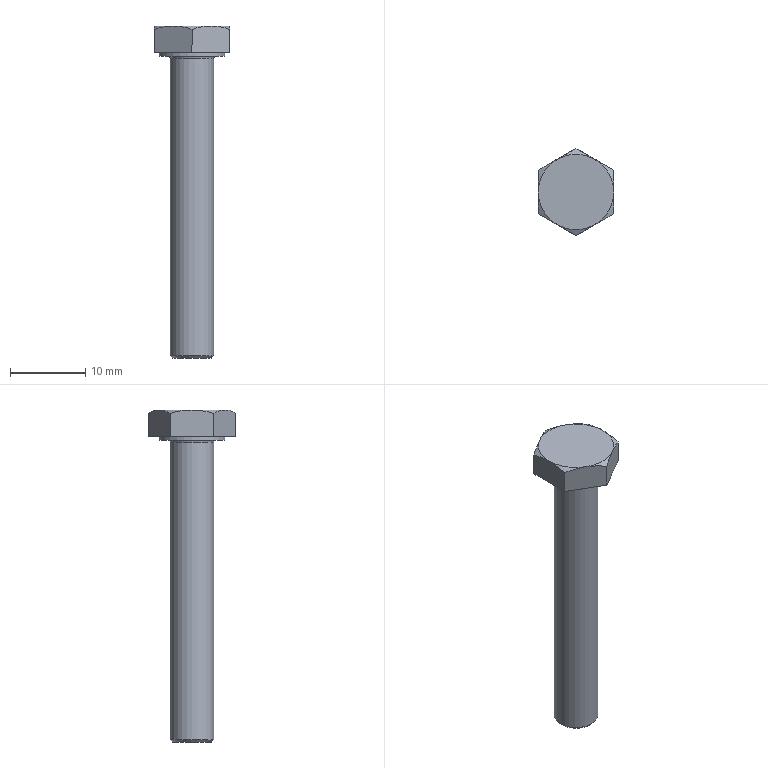Part | NX | features SKETCH 4, EXTRUDE 3, META 3, DATUM_CSYS 2, BLEND 1, CHAMFER 1, LINE 1, SWP104 1, SYMBOLIC_THREAD 1, THREADS 1 | 1 solid | 20 faces | box 10 x 11.547 x 44 mm | volume 1387 mm3 | plane 10 | cone 7 | cylinder 2 | torus 1 | commonest cylinder face diameters 5.795 x1 8.74 x1
STEP:
#1=CARTESIAN_POINT('',(3.147,0.,0.));
#2=VERTEX_POINT('',#1);
#3=CARTESIAN_POINT('',(0.,0.,0.));
#4=DIRECTION('',(0.,0.,1.));
#5=DIRECTION('',(1.,0.,0.));
#6=AXIS2_PLACEMENT_3D('',#3,#4,#5);
#7=CIRCLE('',#6,3.147);
#8=EDGE_CURVE('',#2,#2,#7,.T.);
#9=ORIENTED_EDGE('',*,*,#8,.T.);
#10=EDGE_LOOP('',(#9));
#11=FACE_BOUND('',#10,.T.);
#12=CARTESIAN_POINT('',(4.37,0.,0.));
#13=VERTEX_POINT('',#12);
#14=CARTESIAN_POINT('',(0.,0.,0.));
#15=DIRECTION('',(0.,0.,1.));
#16=DIRECTION('',(1.,0.,0.));
#17=AXIS2_PLACEMENT_3D('',#14,#15,#16);
#18=CIRCLE('',#17,4.37);
#19=EDGE_CURVE('',#13,#13,#18,.T.);
#20=ORIENTED_EDGE('',*,*,#19,.F.);
#21=EDGE_LOOP('',(#20));
#22=FACE_BOUND('',#21,.T.);
#23=CARTESIAN_POINT('',(0.,0.,0.));
#24=DIRECTION('',(0.,0.,1.));
#25=DIRECTION('',(1.,0.,0.));
#26=AXIS2_PLACEMENT_3D('',#23,#24,#25);
#27=PLANE('',#26);
#28=ADVANCED_FACE('',(#11,#22),#27,.F.);
#29=CARTESIAN_POINT('',(5.,2.887,3.553));
#30=VERTEX_POINT('',#29);
#31=CARTESIAN_POINT('',(2.5,4.33,4.));
#32=VERTEX_POINT('',#31);
#33=CARTESIAN_POINT('',(5.,2.887,3.553));
#34=CARTESIAN_POINT('',(4.182,3.359,3.826));
#35=CARTESIAN_POINT('',(3.352,3.838,4.));
#36=CARTESIAN_POINT('',(2.5,4.33,4.));
#37=B_SPLINE_CURVE_WITH_KNOTS('',3,(#33,#34,#35,#36),.UNSPECIFIED.,.F.,.F.,(4,4),(0.000000238,0.002921),.UNSPECIFIED.);
#38=EDGE_CURVE('',#30,#32,#37,.T.);
#39=ORIENTED_EDGE('',*,*,#38,.F.);
#40=CARTESIAN_POINT('',(5.,2.887,0.5));
#41=VERTEX_POINT('',#40);
#42=CARTESIAN_POINT('',(5.,2.887,4.));
#43=DIRECTION('',(0.,0.,-1.));
#44=VECTOR('',#43,1000.);
#45=LINE('',#42,#44);
#46=EDGE_CURVE('',#30,#41,#45,.T.);
#47=ORIENTED_EDGE('',*,*,#46,.T.);
#48=CARTESIAN_POINT('',(0.,5.774,0.5));
#49=VERTEX_POINT('',#48);
#50=CARTESIAN_POINT('',(0.,5.774,0.5));
#51=DIRECTION('',(0.866,-0.5,0.));
#52=VECTOR('',#51,1000.);
#53=LINE('',#50,#52);
#54=EDGE_CURVE('',#49,#41,#53,.T.);
#55=ORIENTED_EDGE('',*,*,#54,.F.);
#56=CARTESIAN_POINT('',(0.,5.774,3.553));
#57=VERTEX_POINT('',#56);
#58=CARTESIAN_POINT('',(0.,5.774,4.));
#59=DIRECTION('',(0.,0.,-1.));
#60=VECTOR('',#59,1000.);
#61=LINE('',#58,#60);
#62=EDGE_CURVE('',#57,#49,#61,.T.);
#63=ORIENTED_EDGE('',*,*,#62,.F.);
#64=CARTESIAN_POINT('',(2.5,4.33,4.));
#65=CARTESIAN_POINT('',(1.651,4.82,4.));
#66=CARTESIAN_POINT('',(0.8159,5.302,3.825));
#67=CARTESIAN_POINT('',(0.,5.774,3.553));
#68=B_SPLINE_CURVE_WITH_KNOTS('',3,(#64,#65,#66,#67),.UNSPECIFIED.,.F.,.F.,(4,4),(0.002921,0.005831),.UNSPECIFIED.);
#69=EDGE_CURVE('',#32,#57,#68,.T.);
#70=ORIENTED_EDGE('',*,*,#69,.F.);
#71=EDGE_LOOP('',(#39,#47,#55,#63,#70));
#72=FACE_BOUND('',#71,.T.);
#73=CARTESIAN_POINT('',(0.,5.774,4.));
#74=DIRECTION('',(0.5,0.866,0.));
#75=DIRECTION('',(-0.866,0.5,0.));
#76=AXIS2_PLACEMENT_3D('',#73,#74,#75);
#77=PLANE('',#76);
#78=ADVANCED_FACE('',(#72),#77,.T.);
#79=CARTESIAN_POINT('',(5.,-2.887,3.553));
#80=VERTEX_POINT('',#79);
#81=CARTESIAN_POINT('',(5.,0.,4.));
#82=VERTEX_POINT('',#81);
#83=CARTESIAN_POINT('',(5.,-2.887,3.553));
#84=CARTESIAN_POINT('',(5.,-1.948,3.824));
#85=CARTESIAN_POINT('',(5.,-0.9756,4.));
#86=CARTESIAN_POINT('',(5.,0.,4.));
#87=B_SPLINE_CURVE_WITH_KNOTS('',3,(#83,#84,#85,#86),.UNSPECIFIED.,.F.,.F.,(4,4),(0.00515,0.008071),.UNSPECIFIED.);
#88=EDGE_CURVE('',#80,#82,#87,.T.);
#89=ORIENTED_EDGE('',*,*,#88,.F.);
#90=CARTESIAN_POINT('',(5.,-2.887,0.5));
#91=VERTEX_POINT('',#90);
#92=CARTESIAN_POINT('',(5.,-2.887,4.));
#93=DIRECTION('',(0.,0.,-1.));
#94=VECTOR('',#93,1000.);
#95=LINE('',#92,#94);
#96=EDGE_CURVE('',#80,#91,#95,.T.);
#97=ORIENTED_EDGE('',*,*,#96,.T.);
#98=CARTESIAN_POINT('',(5.,2.887,0.5));
#99=DIRECTION('',(0.,-1.,0.));
#100=VECTOR('',#99,1000.);
#101=LINE('',#98,#100);
#102=EDGE_CURVE('',#41,#91,#101,.T.);
#103=ORIENTED_EDGE('',*,*,#102,.F.);
#104=ORIENTED_EDGE('',*,*,#46,.F.);
#105=CARTESIAN_POINT('',(5.,0.,4.));
#106=CARTESIAN_POINT('',(5.,0.9762,4.));
#107=CARTESIAN_POINT('',(5.,1.953,3.823));
#108=CARTESIAN_POINT('',(5.,2.887,3.553));
#109=B_SPLINE_CURVE_WITH_KNOTS('',3,(#105,#106,#107,#108),.UNSPECIFIED.,.F.,.F.,(4,4),(0.008071,0.01099),.UNSPECIFIED.);
#110=EDGE_CURVE('',#82,#30,#109,.T.);
#111=ORIENTED_EDGE('',*,*,#110,.F.);
#112=EDGE_LOOP('',(#89,#97,#103,#104,#111));
#113=FACE_BOUND('',#112,.T.);
#114=CARTESIAN_POINT('',(5.,2.887,4.));
#115=DIRECTION('',(1.,0.,0.));
#116=DIRECTION('',(0.,0.,-1.));
#117=AXIS2_PLACEMENT_3D('',#114,#115,#116);
#118=PLANE('',#117);
#119=ADVANCED_FACE('',(#113),#118,.T.);
#120=CARTESIAN_POINT('',(0.,-5.774,3.553));
#121=VERTEX_POINT('',#120);
#122=CARTESIAN_POINT('',(2.5,-4.33,4.));
#123=VERTEX_POINT('',#122);
#124=CARTESIAN_POINT('',(0.,-5.774,3.553));
#125=CARTESIAN_POINT('',(0.8179,-5.301,3.826));
#126=CARTESIAN_POINT('',(1.648,-4.822,4.));
#127=CARTESIAN_POINT('',(2.5,-4.33,4.));
#128=B_SPLINE_CURVE_WITH_KNOTS('',3,(#124,#125,#126,#127),.UNSPECIFIED.,.F.,.F.,(4,4),(0.000000238,0.002921),.UNSPECIFIED.);
#129=EDGE_CURVE('',#121,#123,#128,.T.);
#130=ORIENTED_EDGE('',*,*,#129,.F.);
#131=CARTESIAN_POINT('',(0.,-5.774,0.5));
#132=VERTEX_POINT('',#131);
#133=CARTESIAN_POINT('',(0.,-5.774,4.));
#134=DIRECTION('',(0.,0.,-1.));
#135=VECTOR('',#134,1000.);
#136=LINE('',#133,#135);
#137=EDGE_CURVE('',#121,#132,#136,.T.);
#138=ORIENTED_EDGE('',*,*,#137,.T.);
#139=CARTESIAN_POINT('',(5.,-2.887,0.5));
#140=DIRECTION('',(-0.866,-0.5,0.));
#141=VECTOR('',#140,1000.);
#142=LINE('',#139,#141);
#143=EDGE_CURVE('',#91,#132,#142,.T.);
#144=ORIENTED_EDGE('',*,*,#143,.F.);
#145=ORIENTED_EDGE('',*,*,#96,.F.);
#146=CARTESIAN_POINT('',(2.5,-4.33,4.));
#147=CARTESIAN_POINT('',(3.349,-3.84,4.));
#148=CARTESIAN_POINT('',(4.184,-3.358,3.825));
#149=CARTESIAN_POINT('',(5.,-2.887,3.553));
#150=B_SPLINE_CURVE_WITH_KNOTS('',3,(#146,#147,#148,#149),.UNSPECIFIED.,.F.,.F.,(4,4),(0.002921,0.005831),.UNSPECIFIED.);
#151=EDGE_CURVE('',#123,#80,#150,.T.);
#152=ORIENTED_EDGE('',*,*,#151,.F.);
#153=EDGE_LOOP('',(#130,#138,#144,#145,#152));
#154=FACE_BOUND('',#153,.T.);
#155=CARTESIAN_POINT('',(5.,-2.887,4.));
#156=DIRECTION('',(0.5,-0.866,0.));
#157=DIRECTION('',(0.866,0.5,0.));
#158=AXIS2_PLACEMENT_3D('',#155,#156,#157);
#159=PLANE('',#158);
#160=ADVANCED_FACE('',(#154),#159,.T.);
#161=CARTESIAN_POINT('',(-5.,-2.887,3.553));
#162=VERTEX_POINT('',#161);
#163=CARTESIAN_POINT('',(-2.5,-4.33,4.));
#164=VERTEX_POINT('',#163);
#165=CARTESIAN_POINT('',(-5.,-2.887,3.553));
#166=CARTESIAN_POINT('',(-4.182,-3.359,3.826));
#167=CARTESIAN_POINT('',(-3.352,-3.838,4.));
#168=CARTESIAN_POINT('',(-2.5,-4.33,4.));
#169=B_SPLINE_CURVE_WITH_KNOTS('',3,(#165,#166,#167,#168),.UNSPECIFIED.,.F.,.F.,(4,4),(0.000000238,0.002921),.UNSPECIFIED.);
#170=EDGE_CURVE('',#162,#164,#169,.T.);
#171=ORIENTED_EDGE('',*,*,#170,.F.);
#172=CARTESIAN_POINT('',(-5.,-2.887,0.5));
#173=VERTEX_POINT('',#172);
#174=CARTESIAN_POINT('',(-5.,-2.887,4.));
#175=DIRECTION('',(0.,0.,-1.));
#176=VECTOR('',#175,1000.);
#177=LINE('',#174,#176);
#178=EDGE_CURVE('',#162,#173,#177,.T.);
#179=ORIENTED_EDGE('',*,*,#178,.T.);
#180=CARTESIAN_POINT('',(0.,-5.774,0.5));
#181=DIRECTION('',(-0.866,0.5,0.));
#182=VECTOR('',#181,1000.);
#183=LINE('',#180,#182);
#184=EDGE_CURVE('',#132,#173,#183,.T.);
#185=ORIENTED_EDGE('',*,*,#184,.F.);
#186=ORIENTED_EDGE('',*,*,#137,.F.);
#187=CARTESIAN_POINT('',(-2.5,-4.33,4.));
#188=CARTESIAN_POINT('',(-1.651,-4.82,4.));
#189=CARTESIAN_POINT('',(-0.8159,-5.302,3.825));
#190=CARTESIAN_POINT('',(0.,-5.774,3.553));
#191=B_SPLINE_CURVE_WITH_KNOTS('',3,(#187,#188,#189,#190),.UNSPECIFIED.,.F.,.F.,(4,4),(0.002921,0.005831),.UNSPECIFIED.);
#192=EDGE_CURVE('',#164,#121,#191,.T.);
#193=ORIENTED_EDGE('',*,*,#192,.F.);
#194=EDGE_LOOP('',(#171,#179,#185,#186,#193));
#195=FACE_BOUND('',#194,.T.);
#196=CARTESIAN_POINT('',(0.,-5.774,4.));
#197=DIRECTION('',(-0.5,-0.866,0.));
#198=DIRECTION('',(0.866,-0.5,0.));
#199=AXIS2_PLACEMENT_3D('',#196,#197,#198);
#200=PLANE('',#199);
#201=ADVANCED_FACE('',(#195),#200,.T.);
#202=CARTESIAN_POINT('',(-5.,2.887,3.553));
#203=VERTEX_POINT('',#202);
#204=CARTESIAN_POINT('',(-5.,0.,4.));
#205=VERTEX_POINT('',#204);
#206=CARTESIAN_POINT('',(-5.,0.,4.));
#207=CARTESIAN_POINT('',(-5.,0.9762,4.));
#208=CARTESIAN_POINT('',(-5.,1.953,3.823));
#209=CARTESIAN_POINT('',(-5.,2.887,3.553));
#210=B_SPLINE_CURVE_WITH_KNOTS('',3,(#206,#207,#208,#209),.UNSPECIFIED.,.F.,.F.,(4,4),(0.008071,0.01099),.UNSPECIFIED.);
#211=EDGE_CURVE('',#203,#205,#210,.F.);
#212=ORIENTED_EDGE('',*,*,#211,.F.);
#213=CARTESIAN_POINT('',(-5.,2.887,0.5));
#214=VERTEX_POINT('',#213);
#215=CARTESIAN_POINT('',(-5.,2.887,4.));
#216=DIRECTION('',(0.,0.,-1.));
#217=VECTOR('',#216,1000.);
#218=LINE('',#215,#217);
#219=EDGE_CURVE('',#203,#214,#218,.T.);
#220=ORIENTED_EDGE('',*,*,#219,.T.);
#221=CARTESIAN_POINT('',(-5.,-2.887,0.5));
#222=DIRECTION('',(0.,1.,0.));
#223=VECTOR('',#222,1000.);
#224=LINE('',#221,#223);
#225=EDGE_CURVE('',#173,#214,#224,.T.);
#226=ORIENTED_EDGE('',*,*,#225,.F.);
#227=ORIENTED_EDGE('',*,*,#178,.F.);
#228=CARTESIAN_POINT('',(-5.,-2.887,3.553));
#229=CARTESIAN_POINT('',(-5.,-1.948,3.824));
#230=CARTESIAN_POINT('',(-5.,-0.9756,4.));
#231=CARTESIAN_POINT('',(-5.,0.,4.));
#232=B_SPLINE_CURVE_WITH_KNOTS('',3,(#228,#229,#230,#231),.UNSPECIFIED.,.F.,.F.,(4,4),(0.00515,0.008071),.UNSPECIFIED.);
#233=EDGE_CURVE('',#205,#162,#232,.F.);
#234=ORIENTED_EDGE('',*,*,#233,.F.);
#235=EDGE_LOOP('',(#212,#220,#226,#227,#234));
#236=FACE_BOUND('',#235,.T.);
#237=CARTESIAN_POINT('',(-5.,-2.887,4.));
#238=DIRECTION('',(-1.,0.,0.));
#239=DIRECTION('',(0.,0.,1.));
#240=AXIS2_PLACEMENT_3D('',#237,#238,#239);
#241=PLANE('',#240);
#242=ADVANCED_FACE('',(#236),#241,.T.);
#243=CARTESIAN_POINT('',(-2.5,4.33,4.));
#244=VERTEX_POINT('',#243);
#245=CARTESIAN_POINT('',(0.,5.774,3.553));
#246=CARTESIAN_POINT('',(-0.8179,5.301,3.826));
#247=CARTESIAN_POINT('',(-1.648,4.822,4.));
#248=CARTESIAN_POINT('',(-2.5,4.33,4.));
#249=B_SPLINE_CURVE_WITH_KNOTS('',3,(#245,#246,#247,#248),.UNSPECIFIED.,.F.,.F.,(4,4),(0.000000238,0.002921),.UNSPECIFIED.);
#250=EDGE_CURVE('',#57,#244,#249,.T.);
#251=ORIENTED_EDGE('',*,*,#250,.F.);
#252=ORIENTED_EDGE('',*,*,#62,.T.);
#253=CARTESIAN_POINT('',(-5.,2.887,0.5));
#254=DIRECTION('',(0.866,0.5,0.));
#255=VECTOR('',#254,1000.);
#256=LINE('',#253,#255);
#257=EDGE_CURVE('',#214,#49,#256,.T.);
#258=ORIENTED_EDGE('',*,*,#257,.F.);
#259=ORIENTED_EDGE('',*,*,#219,.F.);
#260=CARTESIAN_POINT('',(-2.5,4.33,4.));
#261=CARTESIAN_POINT('',(-3.349,3.84,4.));
#262=CARTESIAN_POINT('',(-4.184,3.358,3.825));
#263=CARTESIAN_POINT('',(-5.,2.887,3.553));
#264=B_SPLINE_CURVE_WITH_KNOTS('',3,(#260,#261,#262,#263),.UNSPECIFIED.,.F.,.F.,(4,4),(0.002921,0.005831),.UNSPECIFIED.);
#265=EDGE_CURVE('',#244,#203,#264,.T.);
#266=ORIENTED_EDGE('',*,*,#265,.F.);
#267=EDGE_LOOP('',(#251,#252,#258,#259,#266));
#268=FACE_BOUND('',#267,.T.);
#269=CARTESIAN_POINT('',(-5.,2.887,4.));
#270=DIRECTION('',(-0.5,0.866,0.));
#271=DIRECTION('',(-0.866,-0.5,0.));
#272=AXIS2_PLACEMENT_3D('',#269,#270,#271);
#273=PLANE('',#272);
#274=ADVANCED_FACE('',(#268),#273,.T.);
#275=CARTESIAN_POINT('',(4.37,0.,0.5));
#276=VERTEX_POINT('',#275);
#277=CARTESIAN_POINT('',(0.,0.,0.5));
#278=DIRECTION('',(0.,0.,1.));
#279=DIRECTION('',(1.,0.,0.));
#280=AXIS2_PLACEMENT_3D('',#277,#278,#279);
#281=CIRCLE('',#280,4.37);
#282=EDGE_CURVE('',#276,#276,#281,.T.);
#283=ORIENTED_EDGE('',*,*,#282,.T.);
#284=EDGE_LOOP('',(#283));
#285=FACE_BOUND('',#284,.T.);
#286=ORIENTED_EDGE('',*,*,#54,.T.);
#287=ORIENTED_EDGE('',*,*,#102,.T.);
#288=ORIENTED_EDGE('',*,*,#143,.T.);
#289=ORIENTED_EDGE('',*,*,#184,.T.);
#290=ORIENTED_EDGE('',*,*,#225,.T.);
#291=ORIENTED_EDGE('',*,*,#257,.T.);
#292=EDGE_LOOP('',(#286,#287,#288,#289,#290,#291));
#293=FACE_BOUND('',#292,.T.);
#294=CARTESIAN_POINT('',(0.,5.774,0.5));
#295=DIRECTION('',(0.,0.,1.));
#296=DIRECTION('',(1.,0.,0.));
#297=AXIS2_PLACEMENT_3D('',#294,#295,#296);
#298=PLANE('',#297);
#299=ADVANCED_FACE('',(#285,#293),#298,.F.);
#300=ORIENTED_EDGE('',*,*,#282,.F.);
#301=EDGE_LOOP('',(#300));
#302=FACE_BOUND('',#301,.T.);
#303=ORIENTED_EDGE('',*,*,#19,.T.);
#304=EDGE_LOOP('',(#303));
#305=FACE_BOUND('',#304,.T.);
#306=CARTESIAN_POINT('',(0.,0.,0.5));
#307=DIRECTION('',(0.,0.,-1.));
#308=DIRECTION('',(-1.,0.,0.));
#309=AXIS2_PLACEMENT_3D('',#306,#307,#308);
#310=CYLINDRICAL_SURFACE('',#309,4.37);
#311=ADVANCED_FACE('',(#302,#305),#310,.T.);
#312=CARTESIAN_POINT('',(-2.897,0.,-39.71));
#313=VERTEX_POINT('',#312);
#314=CARTESIAN_POINT('',(0.,0.,-39.71));
#315=DIRECTION('',(0.,0.,-1.));
#316=DIRECTION('',(-1.,0.,0.));
#317=AXIS2_PLACEMENT_3D('',#314,#315,#316);
#318=CIRCLE('',#317,2.897);
#319=EDGE_CURVE('',#313,#313,#318,.F.);
#320=ORIENTED_EDGE('',*,*,#319,.T.);
#321=EDGE_LOOP('',(#320));
#322=FACE_BOUND('',#321,.T.);
#323=CARTESIAN_POINT('',(2.897,0.,-0.25));
#324=VERTEX_POINT('',#323);
#325=CARTESIAN_POINT('',(0.,0.,-0.25));
#326=DIRECTION('',(0.,0.,1.));
#327=DIRECTION('',(1.,0.,0.));
#328=AXIS2_PLACEMENT_3D('',#325,#326,#327);
#329=CIRCLE('',#328,2.897);
#330=EDGE_CURVE('',#324,#324,#329,.F.);
#331=ORIENTED_EDGE('',*,*,#330,.T.);
#332=EDGE_LOOP('',(#331));
#333=FACE_BOUND('',#332,.T.);
#334=CARTESIAN_POINT('',(0.,0.,-40.));
#335=DIRECTION('',(0.,0.,1.));
#336=DIRECTION('',(1.,0.,0.));
#337=AXIS2_PLACEMENT_3D('',#334,#335,#336);
#338=CYLINDRICAL_SURFACE('',#337,2.897);
#339=ADVANCED_FACE('',(#322,#333),#338,.T.);
#340=CARTESIAN_POINT('',(-2.608,0.,-40.));
#341=VERTEX_POINT('',#340);
#342=CARTESIAN_POINT('',(0.,0.,-40.));
#343=DIRECTION('',(0.,0.,-1.));
#344=DIRECTION('',(-1.,0.,0.));
#345=AXIS2_PLACEMENT_3D('',#342,#343,#344);
#346=CIRCLE('',#345,2.608);
#347=EDGE_CURVE('',#341,#341,#346,.T.);
#348=ORIENTED_EDGE('',*,*,#347,.T.);
#349=EDGE_LOOP('',(#348));
#350=FACE_BOUND('',#349,.T.);
#351=CARTESIAN_POINT('',(0.,0.,-40.));
#352=DIRECTION('',(0.,0.,-1.));
#353=DIRECTION('',(-1.,0.,0.));
#354=AXIS2_PLACEMENT_3D('',#351,#352,#353);
#355=PLANE('',#354);
#356=ADVANCED_FACE('',(#350),#355,.T.);
#357=ORIENTED_EDGE('',*,*,#211,.T.);
#358=CARTESIAN_POINT('',(0.,0.,4.));
#359=DIRECTION('',(0.,0.,-1.));
#360=DIRECTION('',(-1.,0.,0.));
#361=AXIS2_PLACEMENT_3D('',#358,#359,#360);
#362=CIRCLE('',#361,5.);
#363=EDGE_CURVE('',#205,#244,#362,.T.);
#364=ORIENTED_EDGE('',*,*,#363,.T.);
#365=ORIENTED_EDGE('',*,*,#265,.T.);
#366=EDGE_LOOP('',(#357,#364,#365));
#367=FACE_BOUND('',#366,.T.);
#368=CARTESIAN_POINT('',(0.,0.,4.));
#369=DIRECTION('',(0.,0.,-1.));
#370=DIRECTION('',(-1.,0.,0.));
#371=AXIS2_PLACEMENT_3D('',#368,#369,#370);
#372=CONICAL_SURFACE('',#371,5.,1.047);
#373=ADVANCED_FACE('',(#367),#372,.T.);
#374=ORIENTED_EDGE('',*,*,#69,.T.);
#375=ORIENTED_EDGE('',*,*,#250,.T.);
#376=CARTESIAN_POINT('',(0.,0.,4.));
#377=DIRECTION('',(0.,0.,-1.));
#378=DIRECTION('',(-1.,0.,0.));
#379=AXIS2_PLACEMENT_3D('',#376,#377,#378);
#380=CIRCLE('',#379,5.);
#381=EDGE_CURVE('',#244,#32,#380,.T.);
#382=ORIENTED_EDGE('',*,*,#381,.T.);
#383=EDGE_LOOP('',(#374,#375,#382));
#384=FACE_BOUND('',#383,.T.);
#385=CARTESIAN_POINT('',(0.,0.,4.));
#386=DIRECTION('',(0.,0.,-1.));
#387=DIRECTION('',(-1.,0.,0.));
#388=AXIS2_PLACEMENT_3D('',#385,#386,#387);
#389=CONICAL_SURFACE('',#388,5.,1.047);
#390=ADVANCED_FACE('',(#384),#389,.T.);
#391=ORIENTED_EDGE('',*,*,#170,.T.);
#392=CARTESIAN_POINT('',(0.,0.,4.));
#393=DIRECTION('',(0.,0.,-1.));
#394=DIRECTION('',(-1.,0.,0.));
#395=AXIS2_PLACEMENT_3D('',#392,#393,#394);
#396=CIRCLE('',#395,5.);
#397=EDGE_CURVE('',#164,#205,#396,.T.);
#398=ORIENTED_EDGE('',*,*,#397,.T.);
#399=ORIENTED_EDGE('',*,*,#233,.T.);
#400=EDGE_LOOP('',(#391,#398,#399));
#401=FACE_BOUND('',#400,.T.);
#402=CARTESIAN_POINT('',(0.,0.,4.));
#403=DIRECTION('',(0.,0.,-1.));
#404=DIRECTION('',(-1.,0.,0.));
#405=AXIS2_PLACEMENT_3D('',#402,#403,#404);
#406=CONICAL_SURFACE('',#405,5.,1.047);
#407=ADVANCED_FACE('',(#401),#406,.T.);
#408=ORIENTED_EDGE('',*,*,#129,.T.);
#409=CARTESIAN_POINT('',(0.,0.,4.));
#410=DIRECTION('',(0.,0.,-1.));
#411=DIRECTION('',(-1.,0.,0.));
#412=AXIS2_PLACEMENT_3D('',#409,#410,#411);
#413=CIRCLE('',#412,5.);
#414=EDGE_CURVE('',#123,#164,#413,.T.);
#415=ORIENTED_EDGE('',*,*,#414,.T.);
#416=ORIENTED_EDGE('',*,*,#192,.T.);
#417=EDGE_LOOP('',(#408,#415,#416));
#418=FACE_BOUND('',#417,.T.);
#419=CARTESIAN_POINT('',(0.,0.,4.));
#420=DIRECTION('',(0.,0.,-1.));
#421=DIRECTION('',(-1.,0.,0.));
#422=AXIS2_PLACEMENT_3D('',#419,#420,#421);
#423=CONICAL_SURFACE('',#422,5.,1.047);
#424=ADVANCED_FACE('',(#418),#423,.T.);
#425=ORIENTED_EDGE('',*,*,#151,.T.);
#426=ORIENTED_EDGE('',*,*,#88,.T.);
#427=CARTESIAN_POINT('',(0.,0.,4.));
#428=DIRECTION('',(0.,0.,-1.));
#429=DIRECTION('',(-1.,0.,0.));
#430=AXIS2_PLACEMENT_3D('',#427,#428,#429);
#431=CIRCLE('',#430,5.);
#432=EDGE_CURVE('',#82,#123,#431,.T.);
#433=ORIENTED_EDGE('',*,*,#432,.T.);
#434=EDGE_LOOP('',(#425,#426,#433));
#435=FACE_BOUND('',#434,.T.);
#436=CARTESIAN_POINT('',(0.,0.,4.));
#437=DIRECTION('',(0.,0.,-1.));
#438=DIRECTION('',(-1.,0.,0.));
#439=AXIS2_PLACEMENT_3D('',#436,#437,#438);
#440=CONICAL_SURFACE('',#439,5.,1.047);
#441=ADVANCED_FACE('',(#435),#440,.T.);
#442=ORIENTED_EDGE('',*,*,#110,.T.);
#443=ORIENTED_EDGE('',*,*,#38,.T.);
#444=CARTESIAN_POINT('',(0.,0.,4.));
#445=DIRECTION('',(0.,0.,-1.));
#446=DIRECTION('',(-1.,0.,0.));
#447=AXIS2_PLACEMENT_3D('',#444,#445,#446);
#448=CIRCLE('',#447,5.);
#449=EDGE_CURVE('',#32,#82,#448,.T.);
#450=ORIENTED_EDGE('',*,*,#449,.T.);
#451=EDGE_LOOP('',(#442,#443,#450));
#452=FACE_BOUND('',#451,.T.);
#453=CARTESIAN_POINT('',(0.,0.,4.));
#454=DIRECTION('',(0.,0.,-1.));
#455=DIRECTION('',(-1.,0.,0.));
#456=AXIS2_PLACEMENT_3D('',#453,#454,#455);
#457=CONICAL_SURFACE('',#456,5.,1.047);
#458=ADVANCED_FACE('',(#452),#457,.T.);
#459=ORIENTED_EDGE('',*,*,#363,.F.);
#460=ORIENTED_EDGE('',*,*,#397,.F.);
#461=ORIENTED_EDGE('',*,*,#414,.F.);
#462=ORIENTED_EDGE('',*,*,#432,.F.);
#463=ORIENTED_EDGE('',*,*,#449,.F.);
#464=ORIENTED_EDGE('',*,*,#381,.F.);
#465=EDGE_LOOP('',(#459,#460,#461,#462,#463,#464));
#466=FACE_BOUND('',#465,.T.);
#467=CARTESIAN_POINT('',(0.,5.774,4.));
#468=DIRECTION('',(0.,0.,1.));
#469=DIRECTION('',(1.,0.,0.));
#470=AXIS2_PLACEMENT_3D('',#467,#468,#469);
#471=PLANE('',#470);
#472=ADVANCED_FACE('',(#466),#471,.T.);
#473=ORIENTED_EDGE('',*,*,#8,.F.);
#474=EDGE_LOOP('',(#473));
#475=FACE_BOUND('',#474,.T.);
#476=ORIENTED_EDGE('',*,*,#330,.F.);
#477=EDGE_LOOP('',(#476));
#478=FACE_BOUND('',#477,.T.);
#479=CARTESIAN_POINT('',(0.,0.,-0.25));
#480=DIRECTION('',(0.,0.,1.));
#481=DIRECTION('',(1.,0.,0.));
#482=AXIS2_PLACEMENT_3D('',#479,#480,#481);
#483=TOROIDAL_SURFACE('',#482,3.147,0.25);
#484=ADVANCED_FACE('',(#475,#478),#483,.F.);
#485=ORIENTED_EDGE('',*,*,#319,.F.);
#486=EDGE_LOOP('',(#485));
#487=FACE_BOUND('',#486,.T.);
#488=ORIENTED_EDGE('',*,*,#347,.F.);
#489=EDGE_LOOP('',(#488));
#490=FACE_BOUND('',#489,.T.);
#491=CARTESIAN_POINT('',(0.,0.,-40.));
#492=DIRECTION('',(0.,0.,1.));
#493=DIRECTION('',(1.,0.,0.));
#494=AXIS2_PLACEMENT_3D('',#491,#492,#493);
#495=CONICAL_SURFACE('',#494,2.608,0.7854);
#496=ADVANCED_FACE('',(#487,#490),#495,.T.);
#497=CLOSED_SHELL('',(#28,#78,#119,#160,#201,#242,#274,#299,#311,#339,#356,#373,#390,#407,#424,#441,#458,#472,#484,#496));
#498=MANIFOLD_SOLID_BREP('',#497);
#499=(LENGTH_UNIT()NAMED_UNIT(*)SI_UNIT(.MILLI.,.METRE.));
#500=UNCERTAINTY_MEASURE_WITH_UNIT(LENGTH_MEASURE(0.0508),#499,'','');
#501=(NAMED_UNIT(*)PLANE_ANGLE_UNIT()SI_UNIT($,.RADIAN.));
#502=(NAMED_UNIT(*)SI_UNIT($,.STERADIAN.)SOLID_ANGLE_UNIT());
#503=(GEOMETRIC_REPRESENTATION_CONTEXT(3)GLOBAL_UNCERTAINTY_ASSIGNED_CONTEXT((#500))GLOBAL_UNIT_ASSIGNED_CONTEXT((#499,#501,#502))REPRESENTATION_CONTEXT('',''));
#504=ADVANCED_BREP_SHAPE_REPRESENTATION('',(#498),#503);